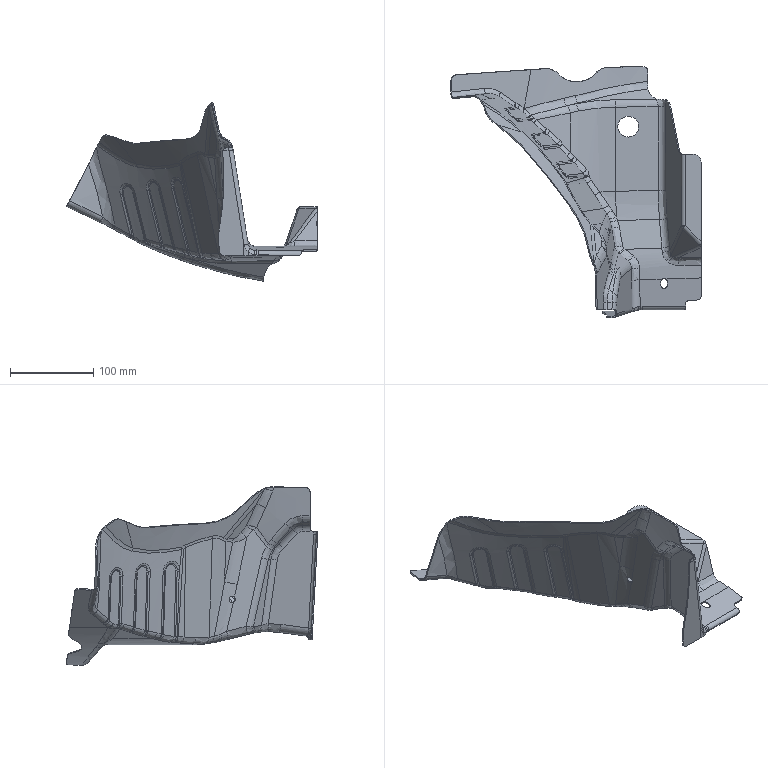Part | 1 solid | 436 faces | box 301.83 x 302.68 x 214.671 mm | volume 147718 mm3 | spline 333 | cylinder 64 | plane 31 | other 6 | sphere 2 | commonest cylinder face diameters 20 x6 23 x5 10 x4 7 x3 9 x3 12 x3